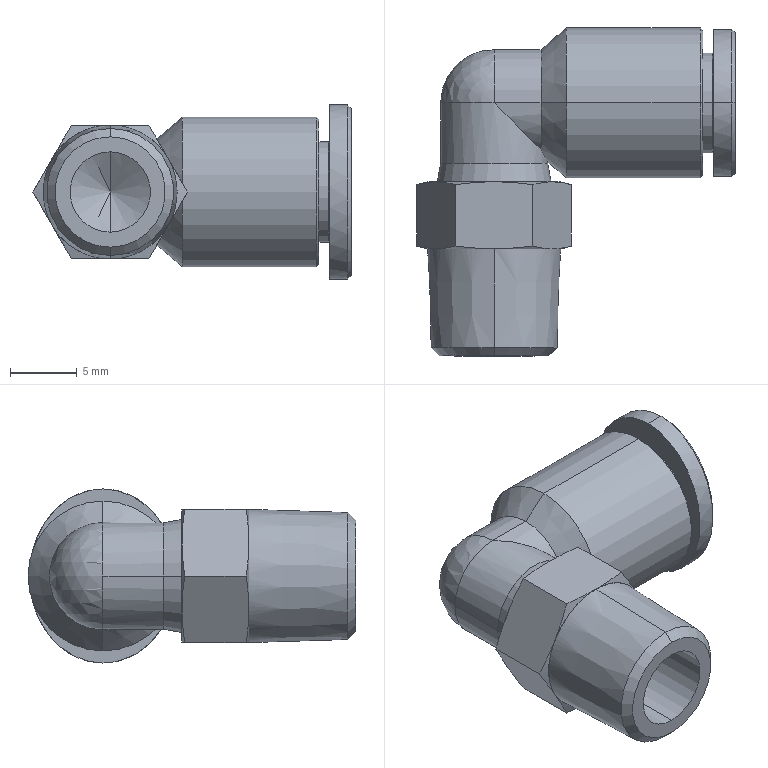Part | STEP file | L-type fitting PL6-01 | 1 solid | 55 faces | box 23.774 x 24.5 x 13 mm | volume 2165 mm3 | cone 24 | cylinder 13 | plane 13 | spline 4 | sphere 1 | commonest cylinder face diameters 8 x5 6 x4 7.5 x2 11.2 x2